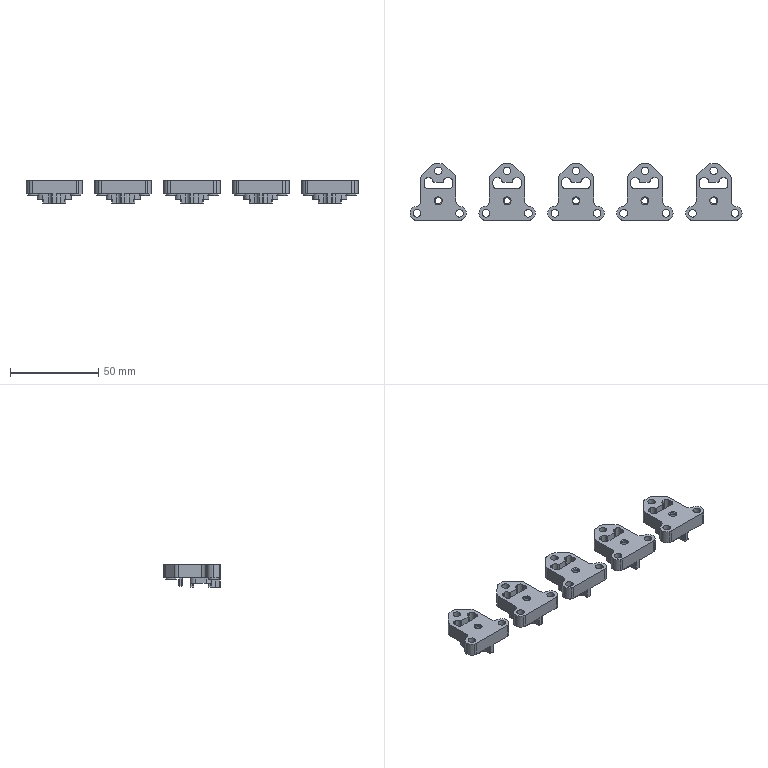Part | 5 solids | 750 faces | box 188 x 32 x 13 mm | volume 20632 mm3 | plane 320 | cylinder 290 | cone 140 | commonest cylinder face diameters 1 x70 6 x70 4 x40 4.3 x30 2.2 x20 6.2 x20